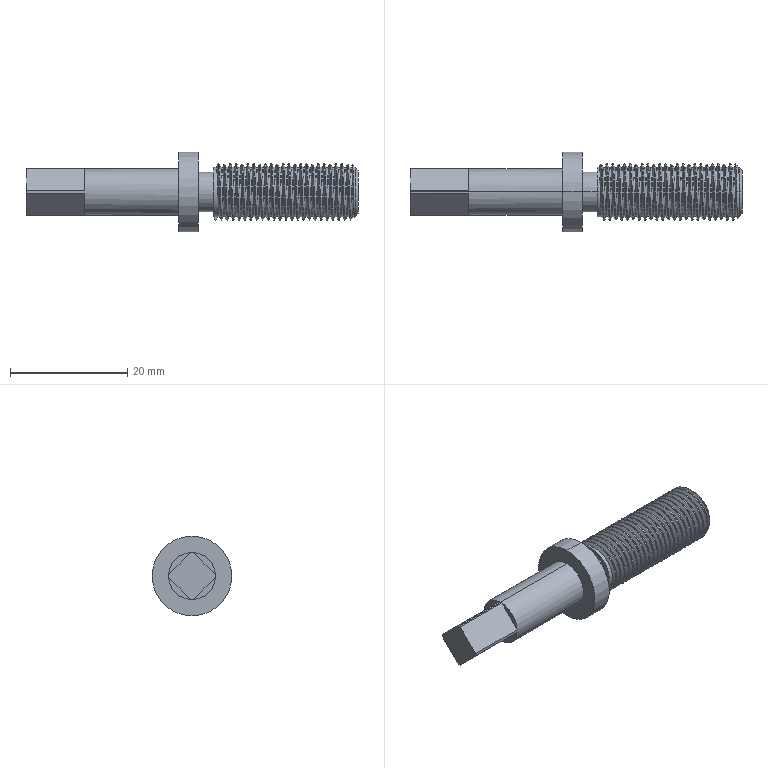Part | SolidWorks | features ICE 5, Chamfer 1, Revolution 1, SweepThread 1 | 1 solid | 77 faces | box 56.6 x 13.6 x 13.6 mm | volume 3300 mm3 | cylinder 55 | plane 14 | spline 6 | cone 2 | commonest cylinder face diameters 8.5 x49 6.8 x2 8 x2 13.6 x2